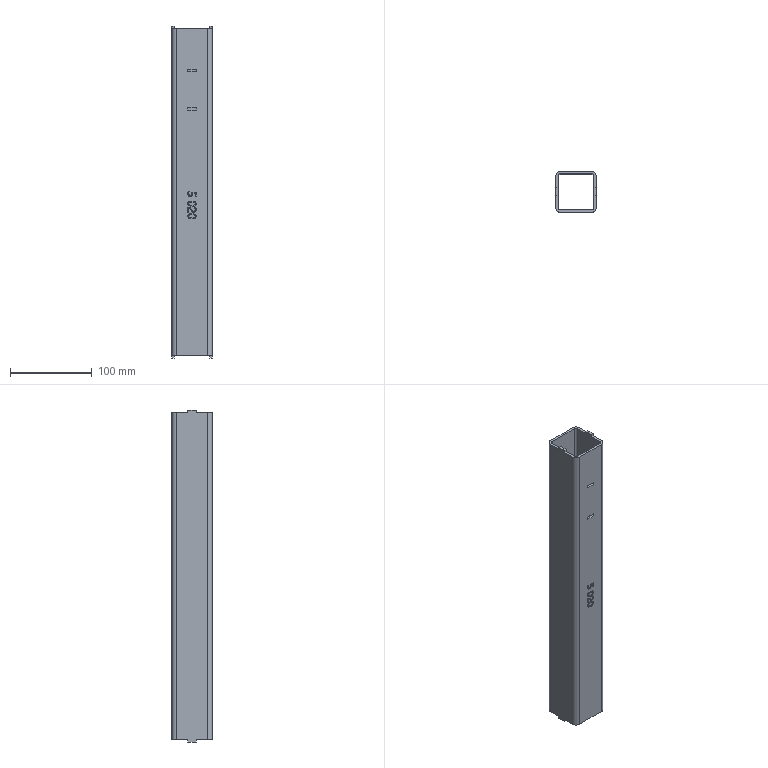Part | SolidWorks | features BaseBody 1 | 1 solid | 89 faces | box 50 x 50 x 406 mm | volume 216470 mm3 | plane 50 | spline 31 | cylinder 8 | commonest cylinder face diameters 6 x4 12 x4